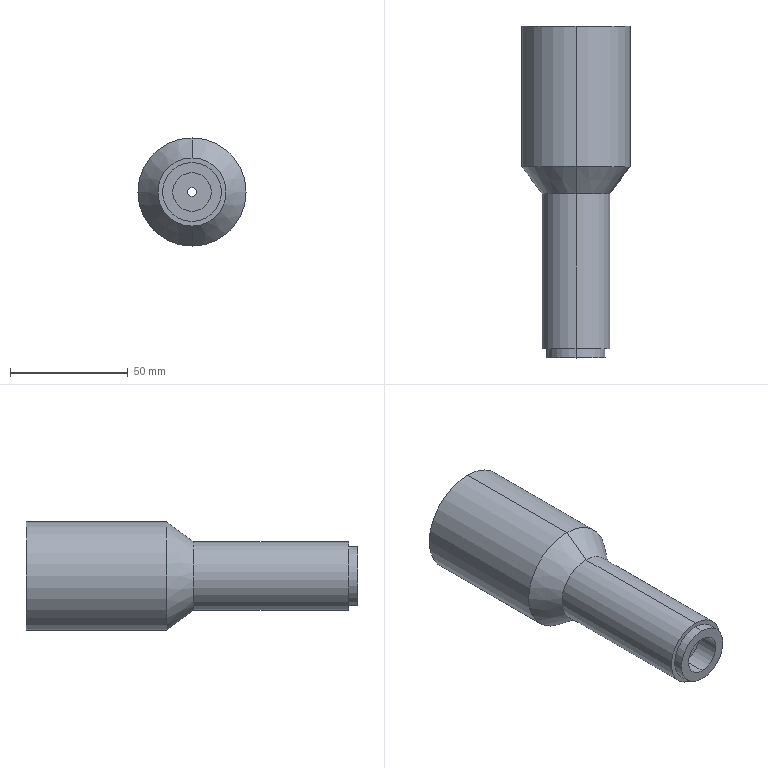Part | STEP file | ASND-0110-Lens | 1 solid | 16 faces | box 46 x 141.1 x 46 mm | volume 154074 mm3 | cylinder 10 | plane 4 | cone 2 | commonest cylinder face diameters 3.74 x2 16.445 x2 25 x2 29 x2 46 x2
STEP:
#1=CARTESIAN_POINT('',(0.,0.,0.));
#2=DIRECTION('',(0.,0.,1.));
#3=DIRECTION('',(1.,0.,0.));
#4=AXIS2_PLACEMENT_3D('',#1,#2,#3);
#5=CARTESIAN_POINT('',(0.,144.654,-23.));
#6=VERTEX_POINT('',#5);
#7=CARTESIAN_POINT('',(0.,144.654,23.));
#8=VERTEX_POINT('',#7);
#9=CARTESIAN_POINT('',(0.,144.654,0.));
#10=DIRECTION('',(0.,-1.,0.));
#11=DIRECTION('',(0.,0.,-1.));
#12=AXIS2_PLACEMENT_3D('',#9,#10,#11);
#13=CIRCLE('',#12,23.);
#14=CARTESIAN_POINT('',(0.,0.,0.));
#15=DIRECTION('',(0.,-1.,0.));
#16=DIRECTION('',(0.,0.,-1.));
#17=AXIS2_PLACEMENT_3D('',#14,#15,#16);
#18=CYLINDRICAL_SURFACE('',#17,23.);
#19=CARTESIAN_POINT('',(0.,-144.654));
#20=DIRECTION('',(1.,0.));
#21=VECTOR('',#20,1.);
#22=LINE('',#19,#21);
#23=(GEOMETRIC_REPRESENTATION_CONTEXT(2)PARAMETRIC_REPRESENTATION_CONTEXT()REPRESENTATION_CONTEXT('',''));
#24=DEFINITIONAL_REPRESENTATION('',(#22),#23);
#25=PCURVE('',#18,#24);
#26=CARTESIAN_POINT('',(23.,144.654,0.));
#27=DIRECTION('',(0.,1.,0.));
#28=DIRECTION('',(0.7071,0.,0.7071));
#29=AXIS2_PLACEMENT_3D('',#26,#27,#28);
#30=PLANE('',#29);
#31=CARTESIAN_POINT('',(-32.527,0.));
#32=CARTESIAN_POINT('',(-4.358,28.169));
#33=CARTESIAN_POINT('',(5.953,-10.311));
#34=CARTESIAN_POINT('',(16.263,-48.79));
#35=CARTESIAN_POINT('',(-22.216,-38.48));
#36=CARTESIAN_POINT('',(-60.696,-28.169));
#37=CARTESIAN_POINT('',(-32.527,0.));
#38=(BOUNDED_CURVE()B_SPLINE_CURVE(2,(#31,#32,#33,#34,#35,#36,#37),.UNSPECIFIED.,.T.,.F.)B_SPLINE_CURVE_WITH_KNOTS((1,2,2,2,2,1),(-2.094,0.,2.094,4.189,6.283,8.378),.UNSPECIFIED.)CURVE()GEOMETRIC_REPRESENTATION_ITEM()RATIONAL_B_SPLINE_CURVE((1.,0.5,1.,0.5,1.,0.5,1.))REPRESENTATION_ITEM(''));
#39=(GEOMETRIC_REPRESENTATION_CONTEXT(2)PARAMETRIC_REPRESENTATION_CONTEXT()REPRESENTATION_CONTEXT('',''));
#40=DEFINITIONAL_REPRESENTATION('',(#38),#39);
#41=PCURVE('',#30,#40);
#42=SURFACE_CURVE('',#13,(#25,#41),.PCURVE_S1.);
#43=EDGE_CURVE('',#6,#8,#42,.T.);
#44=ORIENTED_EDGE('',*,*,#43,.T.);
#45=CARTESIAN_POINT('',(0.,84.922,23.));
#46=VERTEX_POINT('',#45);
#47=CARTESIAN_POINT('',(0.,0.,23.));
#48=DIRECTION('',(0.,-1.,0.));
#49=VECTOR('',#48,1.);
#50=LINE('',#47,#49);
#51=CARTESIAN_POINT('',(3.142,0.));
#52=DIRECTION('',(0.,1.));
#53=VECTOR('',#52,1.);
#54=LINE('',#51,#53);
#55=(GEOMETRIC_REPRESENTATION_CONTEXT(2)PARAMETRIC_REPRESENTATION_CONTEXT()REPRESENTATION_CONTEXT('',''));
#56=DEFINITIONAL_REPRESENTATION('',(#54),#55);
#57=PCURVE('',#18,#56);
#58=CARTESIAN_POINT('',(0.,0.,0.));
#59=DIRECTION('',(0.,-1.,0.));
#60=DIRECTION('',(0.,0.,-1.));
#61=AXIS2_PLACEMENT_3D('',#58,#59,#60);
#62=CYLINDRICAL_SURFACE('',#61,23.);
#63=CARTESIAN_POINT('',(3.142,0.));
#64=DIRECTION('',(0.,1.));
#65=VECTOR('',#64,1.);
#66=LINE('',#63,#65);
#67=(GEOMETRIC_REPRESENTATION_CONTEXT(2)PARAMETRIC_REPRESENTATION_CONTEXT()REPRESENTATION_CONTEXT('',''));
#68=DEFINITIONAL_REPRESENTATION('',(#66),#67);
#69=PCURVE('',#62,#68);
#70=SURFACE_CURVE('',#50,(#57,#69),.PCURVE_S1.);
#71=EDGE_CURVE('',#8,#46,#70,.T.);
#72=ORIENTED_EDGE('',*,*,#71,.T.);
#73=CARTESIAN_POINT('',(0.,84.922,-23.));
#74=VERTEX_POINT('',#73);
#75=CARTESIAN_POINT('',(0.,84.922,0.));
#76=DIRECTION('',(0.,-1.,0.));
#77=DIRECTION('',(0.,0.,-1.));
#78=AXIS2_PLACEMENT_3D('',#75,#76,#77);
#79=CIRCLE('',#78,23.);
#80=CARTESIAN_POINT('',(0.,-84.922));
#81=DIRECTION('',(1.,0.));
#82=VECTOR('',#81,1.);
#83=LINE('',#80,#82);
#84=(GEOMETRIC_REPRESENTATION_CONTEXT(2)PARAMETRIC_REPRESENTATION_CONTEXT()REPRESENTATION_CONTEXT('',''));
#85=DEFINITIONAL_REPRESENTATION('',(#83),#84);
#86=PCURVE('',#18,#85);
#87=CARTESIAN_POINT('',(0.,73.422,0.));
#88=DIRECTION('',(0.,1.,0.));
#89=DIRECTION('',(0.,0.,1.));
#90=AXIS2_PLACEMENT_3D('',#87,#88,#89);
#91=CONICAL_SURFACE('',#90,14.5,0.6365);
#92=CARTESIAN_POINT('',(3.142,11.5));
#93=DIRECTION('',(-1.,0.));
#94=VECTOR('',#93,1.);
#95=LINE('',#92,#94);
#96=(GEOMETRIC_REPRESENTATION_CONTEXT(2)PARAMETRIC_REPRESENTATION_CONTEXT()REPRESENTATION_CONTEXT('',''));
#97=DEFINITIONAL_REPRESENTATION('',(#95),#96);
#98=PCURVE('',#91,#97);
#99=SURFACE_CURVE('',#79,(#86,#98),.PCURVE_S1.);
#100=EDGE_CURVE('',#74,#46,#99,.T.);
#101=ORIENTED_EDGE('',*,*,#100,.F.);
#102=CARTESIAN_POINT('',(0.,0.,-23.));
#103=DIRECTION('',(0.,-1.,0.));
#104=VECTOR('',#103,1.);
#105=LINE('',#102,#104);
#106=CARTESIAN_POINT('',(0.,0.));
#107=DIRECTION('',(0.,1.));
#108=VECTOR('',#107,1.);
#109=LINE('',#106,#108);
#110=(GEOMETRIC_REPRESENTATION_CONTEXT(2)PARAMETRIC_REPRESENTATION_CONTEXT()REPRESENTATION_CONTEXT('',''));
#111=DEFINITIONAL_REPRESENTATION('',(#109),#110);
#112=PCURVE('',#18,#111);
#113=CARTESIAN_POINT('',(6.283,0.));
#114=DIRECTION('',(0.,1.));
#115=VECTOR('',#114,1.);
#116=LINE('',#113,#115);
#117=(GEOMETRIC_REPRESENTATION_CONTEXT(2)PARAMETRIC_REPRESENTATION_CONTEXT()REPRESENTATION_CONTEXT('',''));
#118=DEFINITIONAL_REPRESENTATION('',(#116),#117);
#119=PCURVE('',#62,#118);
#120=SURFACE_CURVE('',#105,(#112,#119),.PCURVE_S1.);
#121=EDGE_CURVE('',#6,#74,#120,.T.);
#122=ORIENTED_EDGE('',*,*,#121,.F.);
#123=EDGE_LOOP('',(#44,#72,#101,#122));
#124=FACE_BOUND('',#123,.T.);
#125=ADVANCED_FACE('',(#124),#18,.T.);
#126=CARTESIAN_POINT('',(0.,73.422,-14.5));
#127=VERTEX_POINT('',#126);
#128=CARTESIAN_POINT('',(0.,73.422,14.5));
#129=VERTEX_POINT('',#128);
#130=CARTESIAN_POINT('',(0.,73.422,0.));
#131=DIRECTION('',(0.,-1.,0.));
#132=DIRECTION('',(0.,0.,-1.));
#133=AXIS2_PLACEMENT_3D('',#130,#131,#132);
#134=CIRCLE('',#133,14.5);
#135=CARTESIAN_POINT('',(3.142,0.));
#136=DIRECTION('',(-1.,0.));
#137=VECTOR('',#136,1.);
#138=LINE('',#135,#137);
#139=(GEOMETRIC_REPRESENTATION_CONTEXT(2)PARAMETRIC_REPRESENTATION_CONTEXT()REPRESENTATION_CONTEXT('',''));
#140=DEFINITIONAL_REPRESENTATION('',(#138),#139);
#141=PCURVE('',#91,#140);
#142=CARTESIAN_POINT('',(0.,0.,0.));
#143=DIRECTION('',(0.,-1.,0.));
#144=DIRECTION('',(0.,0.,-1.));
#145=AXIS2_PLACEMENT_3D('',#142,#143,#144);
#146=CYLINDRICAL_SURFACE('',#145,14.5);
#147=CARTESIAN_POINT('',(0.,-73.422));
#148=DIRECTION('',(1.,0.));
#149=VECTOR('',#148,1.);
#150=LINE('',#147,#149);
#151=(GEOMETRIC_REPRESENTATION_CONTEXT(2)PARAMETRIC_REPRESENTATION_CONTEXT()REPRESENTATION_CONTEXT('',''));
#152=DEFINITIONAL_REPRESENTATION('',(#150),#151);
#153=PCURVE('',#146,#152);
#154=SURFACE_CURVE('',#134,(#141,#153),.PCURVE_S1.);
#155=EDGE_CURVE('',#127,#129,#154,.T.);
#156=ORIENTED_EDGE('',*,*,#155,.F.);
#157=CARTESIAN_POINT('',(0.,73.422,-14.5));
#158=DIRECTION('',(0.,0.8042,-0.5944));
#159=VECTOR('',#158,1.);
#160=LINE('',#157,#159);
#161=CARTESIAN_POINT('',(3.142,0.));
#162=DIRECTION('',(0.,1.));
#163=VECTOR('',#162,1.);
#164=LINE('',#161,#163);
#165=(GEOMETRIC_REPRESENTATION_CONTEXT(2)PARAMETRIC_REPRESENTATION_CONTEXT()REPRESENTATION_CONTEXT('',''));
#166=DEFINITIONAL_REPRESENTATION('',(#164),#165);
#167=PCURVE('',#91,#166);
#168=CARTESIAN_POINT('',(0.,73.422,0.));
#169=DIRECTION('',(0.,1.,0.));
#170=DIRECTION('',(0.,0.,1.));
#171=AXIS2_PLACEMENT_3D('',#168,#169,#170);
#172=CONICAL_SURFACE('',#171,14.5,0.6365);
#173=CARTESIAN_POINT('',(3.142,0.));
#174=DIRECTION('',(0.,1.));
#175=VECTOR('',#174,1.);
#176=LINE('',#173,#175);
#177=(GEOMETRIC_REPRESENTATION_CONTEXT(2)PARAMETRIC_REPRESENTATION_CONTEXT()REPRESENTATION_CONTEXT('',''));
#178=DEFINITIONAL_REPRESENTATION('',(#176),#177);
#179=PCURVE('',#172,#178);
#180=SURFACE_CURVE('',#160,(#167,#179),.PCURVE_S1.);
#181=EDGE_CURVE('',#127,#74,#180,.T.);
#182=ORIENTED_EDGE('',*,*,#181,.T.);
#183=ORIENTED_EDGE('',*,*,#100,.T.);
#184=CARTESIAN_POINT('',(0.,73.422,14.5));
#185=DIRECTION('',(0.,0.8042,0.5944));
#186=VECTOR('',#185,1.);
#187=LINE('',#184,#186);
#188=CARTESIAN_POINT('',(0.,0.));
#189=DIRECTION('',(0.,1.));
#190=VECTOR('',#189,1.);
#191=LINE('',#188,#190);
#192=(GEOMETRIC_REPRESENTATION_CONTEXT(2)PARAMETRIC_REPRESENTATION_CONTEXT()REPRESENTATION_CONTEXT('',''));
#193=DEFINITIONAL_REPRESENTATION('',(#191),#192);
#194=PCURVE('',#91,#193);
#195=CARTESIAN_POINT('',(6.283,0.));
#196=DIRECTION('',(0.,1.));
#197=VECTOR('',#196,1.);
#198=LINE('',#195,#197);
#199=(GEOMETRIC_REPRESENTATION_CONTEXT(2)PARAMETRIC_REPRESENTATION_CONTEXT()REPRESENTATION_CONTEXT('',''));
#200=DEFINITIONAL_REPRESENTATION('',(#198),#199);
#201=PCURVE('',#172,#200);
#202=SURFACE_CURVE('',#187,(#194,#201),.PCURVE_S1.);
#203=EDGE_CURVE('',#129,#46,#202,.T.);
#204=ORIENTED_EDGE('',*,*,#203,.F.);
#205=EDGE_LOOP('',(#156,#182,#183,#204));
#206=FACE_BOUND('',#205,.T.);
#207=ADVANCED_FACE('',(#206),#91,.T.);
#208=ORIENTED_EDGE('',*,*,#155,.T.);
#209=CARTESIAN_POINT('',(0.,7.554,14.5));
#210=VERTEX_POINT('',#209);
#211=CARTESIAN_POINT('',(0.,0.,14.5));
#212=DIRECTION('',(0.,-1.,0.));
#213=VECTOR('',#212,1.);
#214=LINE('',#211,#213);
#215=CARTESIAN_POINT('',(3.142,0.));
#216=DIRECTION('',(0.,1.));
#217=VECTOR('',#216,1.);
#218=LINE('',#215,#217);
#219=(GEOMETRIC_REPRESENTATION_CONTEXT(2)PARAMETRIC_REPRESENTATION_CONTEXT()REPRESENTATION_CONTEXT('',''));
#220=DEFINITIONAL_REPRESENTATION('',(#218),#219);
#221=PCURVE('',#146,#220);
#222=CARTESIAN_POINT('',(0.,0.,0.));
#223=DIRECTION('',(0.,-1.,0.));
#224=DIRECTION('',(0.,0.,-1.));
#225=AXIS2_PLACEMENT_3D('',#222,#223,#224);
#226=CYLINDRICAL_SURFACE('',#225,14.5);
#227=CARTESIAN_POINT('',(3.142,0.));
#228=DIRECTION('',(0.,1.));
#229=VECTOR('',#228,1.);
#230=LINE('',#227,#229);
#231=(GEOMETRIC_REPRESENTATION_CONTEXT(2)PARAMETRIC_REPRESENTATION_CONTEXT()REPRESENTATION_CONTEXT('',''));
#232=DEFINITIONAL_REPRESENTATION('',(#230),#231);
#233=PCURVE('',#226,#232);
#234=SURFACE_CURVE('',#214,(#221,#233),.PCURVE_S1.);
#235=EDGE_CURVE('',#129,#210,#234,.T.);
#236=ORIENTED_EDGE('',*,*,#235,.T.);
#237=CARTESIAN_POINT('',(0.,7.554,-14.5));
#238=VERTEX_POINT('',#237);
#239=CARTESIAN_POINT('',(0.,7.554,0.));
#240=DIRECTION('',(0.,-1.,0.));
#241=DIRECTION('',(0.,0.,-1.));
#242=AXIS2_PLACEMENT_3D('',#239,#240,#241);
#243=CIRCLE('',#242,14.5);
#244=CARTESIAN_POINT('',(0.,-7.554));
#245=DIRECTION('',(1.,0.));
#246=VECTOR('',#245,1.);
#247=LINE('',#244,#246);
#248=(GEOMETRIC_REPRESENTATION_CONTEXT(2)PARAMETRIC_REPRESENTATION_CONTEXT()REPRESENTATION_CONTEXT('',''));
#249=DEFINITIONAL_REPRESENTATION('',(#247),#248);
#250=PCURVE('',#146,#249);
#251=CARTESIAN_POINT('',(14.5,7.554,0.));
#252=DIRECTION('',(0.,-1.,0.));
#253=DIRECTION('',(0.7071,0.,0.7071));
#254=AXIS2_PLACEMENT_3D('',#251,#252,#253);
#255=PLANE('',#254);
#256=CARTESIAN_POINT('',(-10.253,10.253));
#257=DIRECTION('',(-0.7071,-0.7071));
#258=AXIS2_PLACEMENT_2D('',#256,#257);
#259=CIRCLE('',#258,14.5);
#260=(GEOMETRIC_REPRESENTATION_CONTEXT(2)PARAMETRIC_REPRESENTATION_CONTEXT()REPRESENTATION_CONTEXT('',''));
#261=DEFINITIONAL_REPRESENTATION('',(#259),#260);
#262=PCURVE('',#255,#261);
#263=SURFACE_CURVE('',#243,(#250,#262),.PCURVE_S1.);
#264=EDGE_CURVE('',#238,#210,#263,.T.);
#265=ORIENTED_EDGE('',*,*,#264,.F.);
#266=CARTESIAN_POINT('',(0.,0.,-14.5));
#267=DIRECTION('',(0.,-1.,0.));
#268=VECTOR('',#267,1.);
#269=LINE('',#266,#268);
#270=CARTESIAN_POINT('',(0.,0.));
#271=DIRECTION('',(0.,1.));
#272=VECTOR('',#271,1.);
#273=LINE('',#270,#272);
#274=(GEOMETRIC_REPRESENTATION_CONTEXT(2)PARAMETRIC_REPRESENTATION_CONTEXT()REPRESENTATION_CONTEXT('',''));
#275=DEFINITIONAL_REPRESENTATION('',(#273),#274);
#276=PCURVE('',#146,#275);
#277=CARTESIAN_POINT('',(6.283,0.));
#278=DIRECTION('',(0.,1.));
#279=VECTOR('',#278,1.);
#280=LINE('',#277,#279);
#281=(GEOMETRIC_REPRESENTATION_CONTEXT(2)PARAMETRIC_REPRESENTATION_CONTEXT()REPRESENTATION_CONTEXT('',''));
#282=DEFINITIONAL_REPRESENTATION('',(#280),#281);
#283=PCURVE('',#226,#282);
#284=SURFACE_CURVE('',#269,(#276,#283),.PCURVE_S1.);
#285=EDGE_CURVE('',#127,#238,#284,.T.);
#286=ORIENTED_EDGE('',*,*,#285,.F.);
#287=EDGE_LOOP('',(#208,#236,#265,#286));
#288=FACE_BOUND('',#287,.T.);
#289=ADVANCED_FACE('',(#288),#146,.T.);
#290=CARTESIAN_POINT('',(0.,7.554,-12.5));
#291=VERTEX_POINT('',#290);
#292=CARTESIAN_POINT('',(0.,7.554,12.5));
#293=VERTEX_POINT('',#292);
#294=CARTESIAN_POINT('',(0.,7.554,0.));
#295=DIRECTION('',(0.,-1.,0.));
#296=DIRECTION('',(0.,0.,-1.));
#297=AXIS2_PLACEMENT_3D('',#294,#295,#296);
#298=CIRCLE('',#297,12.5);
#299=CARTESIAN_POINT('',(0.,0.,0.));
#300=DIRECTION('',(0.,-1.,0.));
#301=DIRECTION('',(0.,0.,-1.));
#302=AXIS2_PLACEMENT_3D('',#299,#300,#301);
#303=CYLINDRICAL_SURFACE('',#302,12.5);
#304=CARTESIAN_POINT('',(0.,-7.554));
#305=DIRECTION('',(1.,0.));
#306=VECTOR('',#305,1.);
#307=LINE('',#304,#306);
#308=(GEOMETRIC_REPRESENTATION_CONTEXT(2)PARAMETRIC_REPRESENTATION_CONTEXT()REPRESENTATION_CONTEXT('',''));
#309=DEFINITIONAL_REPRESENTATION('',(#307),#308);
#310=PCURVE('',#303,#309);
#311=CARTESIAN_POINT('',(-10.253,10.253));
#312=DIRECTION('',(-0.7071,-0.7071));
#313=AXIS2_PLACEMENT_2D('',#311,#312);
#314=CIRCLE('',#313,12.5);
#315=(GEOMETRIC_REPRESENTATION_CONTEXT(2)PARAMETRIC_REPRESENTATION_CONTEXT()REPRESENTATION_CONTEXT('',''));
#316=DEFINITIONAL_REPRESENTATION('',(#314),#315);
#317=PCURVE('',#255,#316);
#318=SURFACE_CURVE('',#298,(#310,#317),.PCURVE_S1.);
#319=EDGE_CURVE('',#291,#293,#318,.T.);
#320=ORIENTED_EDGE('',*,*,#319,.T.);
#321=CARTESIAN_POINT('',(0.,3.554,12.5));
#322=VERTEX_POINT('',#321);
#323=CARTESIAN_POINT('',(0.,0.,12.5));
#324=DIRECTION('',(0.,-1.,0.));
#325=VECTOR('',#324,1.);
#326=LINE('',#323,#325);
#327=CARTESIAN_POINT('',(3.142,0.));
#328=DIRECTION('',(0.,1.));
#329=VECTOR('',#328,1.);
#330=LINE('',#327,#329);
#331=(GEOMETRIC_REPRESENTATION_CONTEXT(2)PARAMETRIC_REPRESENTATION_CONTEXT()REPRESENTATION_CONTEXT('',''));
#332=DEFINITIONAL_REPRESENTATION('',(#330),#331);
#333=PCURVE('',#303,#332);
#334=CARTESIAN_POINT('',(0.,0.,0.));
#335=DIRECTION('',(0.,-1.,0.));
#336=DIRECTION('',(0.,0.,-1.));
#337=AXIS2_PLACEMENT_3D('',#334,#335,#336);
#338=CYLINDRICAL_SURFACE('',#337,12.5);
#339=CARTESIAN_POINT('',(3.142,0.));
#340=DIRECTION('',(0.,1.));
#341=VECTOR('',#340,1.);
#342=LINE('',#339,#341);
#343=(GEOMETRIC_REPRESENTATION_CONTEXT(2)PARAMETRIC_REPRESENTATION_CONTEXT()REPRESENTATION_CONTEXT('',''));
#344=DEFINITIONAL_REPRESENTATION('',(#342),#343);
#345=PCURVE('',#338,#344);
#346=SURFACE_CURVE('',#326,(#333,#345),.PCURVE_S1.);
#347=EDGE_CURVE('',#293,#322,#346,.T.);
#348=ORIENTED_EDGE('',*,*,#347,.T.);
#349=CARTESIAN_POINT('',(0.,3.554,-12.5));
#350=VERTEX_POINT('',#349);
#351=CARTESIAN_POINT('',(0.,3.554,0.));
#352=DIRECTION('',(0.,-1.,0.));
#353=DIRECTION('',(0.,0.,-1.));
#354=AXIS2_PLACEMENT_3D('',#351,#352,#353);
#355=CIRCLE('',#354,12.5);
#356=CARTESIAN_POINT('',(0.,-3.554));
#357=DIRECTION('',(1.,0.));
#358=VECTOR('',#357,1.);
#359=LINE('',#356,#358);
#360=(GEOMETRIC_REPRESENTATION_CONTEXT(2)PARAMETRIC_REPRESENTATION_CONTEXT()REPRESENTATION_CONTEXT('',''));
#361=DEFINITIONAL_REPRESENTATION('',(#359),#360);
#362=PCURVE('',#303,#361);
#363=CARTESIAN_POINT('',(12.5,3.554,0.));
#364=DIRECTION('',(0.,-1.,0.));
#365=DIRECTION('',(0.7071,0.,0.7071));
#366=AXIS2_PLACEMENT_3D('',#363,#364,#365);
#367=PLANE('',#366);
#368=CARTESIAN_POINT('',(-8.839,8.839));
#369=DIRECTION('',(-0.7071,-0.7071));
#370=AXIS2_PLACEMENT_2D('',#368,#369);
#371=CIRCLE('',#370,12.5);
#372=(GEOMETRIC_REPRESENTATION_CONTEXT(2)PARAMETRIC_REPRESENTATION_CONTEXT()REPRESENTATION_CONTEXT('',''));
#373=DEFINITIONAL_REPRESENTATION('',(#371),#372);
#374=PCURVE('',#367,#373);
#375=SURFACE_CURVE('',#355,(#362,#374),.PCURVE_S1.);
#376=EDGE_CURVE('',#350,#322,#375,.T.);
#377=ORIENTED_EDGE('',*,*,#376,.F.);
#378=CARTESIAN_POINT('',(0.,0.,-12.5));
#379=DIRECTION('',(0.,-1.,0.));
#380=VECTOR('',#379,1.);
#381=LINE('',#378,#380);
#382=CARTESIAN_POINT('',(0.,0.));
#383=DIRECTION('',(0.,1.));
#384=VECTOR('',#383,1.);
#385=LINE('',#382,#384);
#386=(GEOMETRIC_REPRESENTATION_CONTEXT(2)PARAMETRIC_REPRESENTATION_CONTEXT()REPRESENTATION_CONTEXT('',''));
#387=DEFINITIONAL_REPRESENTATION('',(#385),#386);
#388=PCURVE('',#303,#387);
#389=CARTESIAN_POINT('',(6.283,0.));
#390=DIRECTION('',(0.,1.));
#391=VECTOR('',#390,1.);
#392=LINE('',#389,#391);
#393=(GEOMETRIC_REPRESENTATION_CONTEXT(2)PARAMETRIC_REPRESENTATION_CONTEXT()REPRESENTATION_CONTEXT('',''));
#394=DEFINITIONAL_REPRESENTATION('',(#392),#393);
#395=PCURVE('',#338,#394);
#396=SURFACE_CURVE('',#381,(#388,#395),.PCURVE_S1.);
#397=EDGE_CURVE('',#291,#350,#396,.T.);
#398=ORIENTED_EDGE('',*,*,#397,.F.);
#399=EDGE_LOOP('',(#320,#348,#377,#398));
#400=FACE_BOUND('',#399,.T.);
#401=ADVANCED_FACE('',(#400),#303,.T.);
#402=CARTESIAN_POINT('',(0.,13.654,-8.222));
#403=VERTEX_POINT('',#402);
#404=CARTESIAN_POINT('',(0.,3.554,-8.222));
#405=VERTEX_POINT('',#404);
#406=CARTESIAN_POINT('',(0.,0.,-8.222));
#407=DIRECTION('',(0.,-1.,0.));
#408=VECTOR('',#407,1.);
#409=LINE('',#406,#408);
#410=CARTESIAN_POINT('',(0.,0.,0.));
#411=DIRECTION('',(0.,-1.,0.));
#412=DIRECTION('',(0.,0.,-1.));
#413=AXIS2_PLACEMENT_3D('',#410,#411,#412);
#414=CYLINDRICAL_SURFACE('',#413,8.222);
#415=CARTESIAN_POINT('',(6.283,0.));
#416=DIRECTION('',(0.,1.));
#417=VECTOR('',#416,1.);
#418=LINE('',#415,#417);
#419=(GEOMETRIC_REPRESENTATION_CONTEXT(2)PARAMETRIC_REPRESENTATION_CONTEXT()REPRESENTATION_CONTEXT('',''));
#420=DEFINITIONAL_REPRESENTATION('',(#418),#419);
#421=PCURVE('',#414,#420);
#422=CARTESIAN_POINT('',(0.,0.,0.));
#423=DIRECTION('',(0.,-1.,0.));
#424=DIRECTION('',(0.,0.,-1.));
#425=AXIS2_PLACEMENT_3D('',#422,#423,#424);
#426=CYLINDRICAL_SURFACE('',#425,8.222);
#427=CARTESIAN_POINT('',(0.,0.));
#428=DIRECTION('',(0.,1.));
#429=VECTOR('',#428,1.);
#430=LINE('',#427,#429);
#431=(GEOMETRIC_REPRESENTATION_CONTEXT(2)PARAMETRIC_REPRESENTATION_CONTEXT()REPRESENTATION_CONTEXT('',''));
#432=DEFINITIONAL_REPRESENTATION('',(#430),#431);
#433=PCURVE('',#426,#432);
#434=SURFACE_CURVE('',#409,(#421,#433),.PCURVE_S1.);
#435=EDGE_CURVE('',#403,#405,#434,.T.);
#436=ORIENTED_EDGE('',*,*,#435,.T.);
#437=CARTESIAN_POINT('',(0.,3.554,8.222));
#438=VERTEX_POINT('',#437);
#439=CARTESIAN_POINT('',(0.,3.554,0.));
#440=DIRECTION('',(0.,-1.,0.));
#441=DIRECTION('',(0.,0.,-1.));
#442=AXIS2_PLACEMENT_3D('',#439,#440,#441);
#443=CIRCLE('',#442,8.222);
#444=CARTESIAN_POINT('',(0.,-3.554));
#445=DIRECTION('',(1.,0.));
#446=VECTOR('',#445,1.);
#447=LINE('',#444,#446);
#448=(GEOMETRIC_REPRESENTATION_CONTEXT(2)PARAMETRIC_REPRESENTATION_CONTEXT()REPRESENTATION_CONTEXT('',''));
#449=DEFINITIONAL_REPRESENTATION('',(#447),#448);
#450=PCURVE('',#414,#449);
#451=CARTESIAN_POINT('',(-8.839,8.839));
#452=DIRECTION('',(-0.7071,-0.7071));
#453=AXIS2_PLACEMENT_2D('',#451,#452);
#454=CIRCLE('',#453,8.222);
#455=(GEOMETRIC_REPRESENTATION_CONTEXT(2)PARAMETRIC_REPRESENTATION_CONTEXT()REPRESENTATION_CONTEXT('',''));
#456=DEFINITIONAL_REPRESENTATION('',(#454),#455);
#457=PCURVE('',#367,#456);
#458=SURFACE_CURVE('',#443,(#450,#457),.PCURVE_S1.);
#459=EDGE_CURVE('',#438,#405,#458,.T.);
#460=ORIENTED_EDGE('',*,*,#459,.F.);
#461=CARTESIAN_POINT('',(0.,13.654,8.222));
#462=VERTEX_POINT('',#461);
#463=CARTESIAN_POINT('',(0.,0.,8.222));
#464=DIRECTION('',(0.,-1.,0.));
#465=VECTOR('',#464,1.);
#466=LINE('',#463,#465);
#467=CARTESIAN_POINT('',(3.142,0.));
#468=DIRECTION('',(0.,1.));
#469=VECTOR('',#468,1.);
#470=LINE('',#467,#469);
#471=(GEOMETRIC_REPRESENTATION_CONTEXT(2)PARAMETRIC_REPRESENTATION_CONTEXT()REPRESENTATION_CONTEXT('',''));
#472=DEFINITIONAL_REPRESENTATION('',(#470),#471);
#473=PCURVE('',#414,#472);
#474=CARTESIAN_POINT('',(3.142,0.));
#475=DIRECTION('',(0.,1.));
#476=VECTOR('',#475,1.);
#477=LINE('',#474,#476);
#478=(GEOMETRIC_REPRESENTATION_CONTEXT(2)PARAMETRIC_REPRESENTATION_CONTEXT()REPRESENTATION_CONTEXT('',''));
#479=DEFINITIONAL_REPRESENTATION('',(#477),#478);
#480=PCURVE('',#426,#479);
#481=SURFACE_CURVE('',#466,(#473,#480),.PCURVE_S1.);
#482=EDGE_CURVE('',#462,#438,#481,.T.);
#483=ORIENTED_EDGE('',*,*,#482,.F.);
#484=CARTESIAN_POINT('',(0.,13.654,0.));
#485=DIRECTION('',(0.,-1.,0.));
#486=DIRECTION('',(0.,0.,-1.));
#487=AXIS2_PLACEMENT_3D('',#484,#485,#486);
#488=CIRCLE('',#487,8.222);
#489=CARTESIAN_POINT('',(0.,-13.654));
#490=DIRECTION('',(1.,0.));
#491=VECTOR('',#490,1.);
#492=LINE('',#489,#491);
#493=(GEOMETRIC_REPRESENTATION_CONTEXT(2)PARAMETRIC_REPRESENTATION_CONTEXT()REPRESENTATION_CONTEXT('',''));
#494=DEFINITIONAL_REPRESENTATION('',(#492),#493);
#495=PCURVE('',#414,#494);
#496=CARTESIAN_POINT('',(1.87,13.654,0.));
#497=DIRECTION('',(0.,-1.,0.));
#498=DIRECTION('',(0.7071,0.,0.7071));
#499=AXIS2_PLACEMENT_3D('',#496,#497,#498);
#500=PLANE('',#499);
#501=CARTESIAN_POINT('',(-1.322,1.322));
#502=DIRECTION('',(-0.7071,-0.7071));
#503=AXIS2_PLACEMENT_2D('',#501,#502);
#504=CIRCLE('',#503,8.222);
#505=(GEOMETRIC_REPRESENTATION_CONTEXT(2)PARAMETRIC_REPRESENTATION_CONTEXT()REPRESENTATION_CONTEXT('',''));
#506=DEFINITIONAL_REPRESENTATION('',(#504),#505);
#507=PCURVE('',#500,#506);
#508=SURFACE_CURVE('',#488,(#495,#507),.PCURVE_S1.);
#509=EDGE_CURVE('',#462,#403,#508,.T.);
#510=ORIENTED_EDGE('',*,*,#509,.T.);
#511=EDGE_LOOP('',(#436,#460,#483,#510));
#512=FACE_BOUND('',#511,.F.);
#513=ADVANCED_FACE('',(#512),#414,.F.);
#514=CARTESIAN_POINT('',(0.,144.654,-1.87));
#515=VERTEX_POINT('',#514);
#516=CARTESIAN_POINT('',(0.,13.654,-1.87));
#517=VERTEX_POINT('',#516);
#518=CARTESIAN_POINT('',(0.,0.,-1.87));
#519=DIRECTION('',(0.,-1.,0.));
#520=VECTOR('',#519,1.);
#521=LINE('',#518,#520);
#522=CARTESIAN_POINT('',(0.,0.,0.));
#523=DIRECTION('',(0.,-1.,0.));
#524=DIRECTION('',(0.,0.,-1.));
#525=AXIS2_PLACEMENT_3D('',#522,#523,#524);
#526=CYLINDRICAL_SURFACE('',#525,1.87);
#527=CARTESIAN_POINT('',(6.283,0.));
#528=DIRECTION('',(0.,1.));
#529=VECTOR('',#528,1.);
#530=LINE('',#527,#529);
#531=(GEOMETRIC_REPRESENTATION_CONTEXT(2)PARAMETRIC_REPRESENTATION_CONTEXT()REPRESENTATION_CONTEXT('',''));
#532=DEFINITIONAL_REPRESENTATION('',(#530),#531);
#533=PCURVE('',#526,#532);
#534=CARTESIAN_POINT('',(0.,0.,0.));
#535=DIRECTION('',(0.,-1.,0.));
#536=DIRECTION('',(0.,0.,-1.));
#537=AXIS2_PLACEMENT_3D('',#534,#535,#536);
#538=CYLINDRICAL_SURFACE('',#537,1.87);
#539=CARTESIAN_POINT('',(0.,0.));
#540=DIRECTION('',(0.,1.));
#541=VECTOR('',#540,1.);
#542=LINE('',#539,#541);
#543=(GEOMETRIC_REPRESENTATION_CONTEXT(2)PARAMETRIC_REPRESENTATION_CONTEXT()REPRESENTATION_CONTEXT('',''));
#544=DEFINITIONAL_REPRESENTATION('',(#542),#543);
#545=PCURVE('',#538,#544);
#546=SURFACE_CURVE('',#521,(#533,#545),.PCURVE_S1.);
#547=EDGE_CURVE('',#515,#517,#546,.T.);
#548=ORIENTED_EDGE('',*,*,#547,.T.);
#549=CARTESIAN_POINT('',(0.,13.654,1.87));
#550=VERTEX_POINT('',#549);
#551=CARTESIAN_POINT('',(0.,13.654,0.));
#552=DIRECTION('',(0.,-1.,0.));
#553=DIRECTION('',(0.,0.,-1.));
#554=AXIS2_PLACEMENT_3D('',#551,#552,#553);
#555=CIRCLE('',#554,1.87);
#556=CARTESIAN_POINT('',(0.,-13.654));
#557=DIRECTION('',(1.,0.));
#558=VECTOR('',#557,1.);
#559=LINE('',#556,#558);
#560=(GEOMETRIC_REPRESENTATION_CONTEXT(2)PARAMETRIC_REPRESENTATION_CONTEXT()REPRESENTATION_CONTEXT('',''));
#561=DEFINITIONAL_REPRESENTATION('',(#559),#560);
#562=PCURVE('',#526,#561);
#563=CARTESIAN_POINT('',(-1.322,1.322));
#564=DIRECTION('',(-0.7071,-0.7071));
#565=AXIS2_PLACEMENT_2D('',#563,#564);
#566=CIRCLE('',#565,1.87);
#567=(GEOMETRIC_REPRESENTATION_CONTEXT(2)PARAMETRIC_REPRESENTATION_CONTEXT()REPRESENTATION_CONTEXT('',''));
#568=DEFINITIONAL_REPRESENTATION('',(#566),#567);
#569=PCURVE('',#500,#568);
#570=SURFACE_CURVE('',#555,(#562,#569),.PCURVE_S1.);
#571=EDGE_CURVE('',#550,#517,#570,.T.);
#572=ORIENTED_EDGE('',*,*,#571,.F.);
#573=CARTESIAN_POINT('',(0.,144.654,1.87));
#574=VERTEX_POINT('',#573);
#575=CARTESIAN_POINT('',(0.,0.,1.87));
#576=DIRECTION('',(0.,-1.,0.));
#577=VECTOR('',#576,1.);
#578=LINE('',#575,#577);
#579=CARTESIAN_POINT('',(3.142,0.));
#580=DIRECTION('',(0.,1.));
#581=VECTOR('',#580,1.);
#582=LINE('',#579,#581);
#583=(GEOMETRIC_REPRESENTATION_CONTEXT(2)PARAMETRIC_REPRESENTATION_CONTEXT()REPRESENTATION_CONTEXT('',''));
#584=DEFINITIONAL_REPRESENTATION('',(#582),#583);
#585=PCURVE('',#526,#584);
#586=CARTESIAN_POINT('',(3.142,0.));
#587=DIRECTION('',(0.,1.));
#588=VECTOR('',#587,1.);
#589=LINE('',#586,#588);
#590=(GEOMETRIC_REPRESENTATION_CONTEXT(2)PARAMETRIC_REPRESENTATION_CONTEXT()REPRESENTATION_CONTEXT('',''));
#591=DEFINITIONAL_REPRESENTATION('',(#589),#590);
#592=PCURVE('',#538,#591);
#593=SURFACE_CURVE('',#578,(#585,#592),.PCURVE_S1.);
#594=EDGE_CURVE('',#574,#550,#593,.T.);
#595=ORIENTED_EDGE('',*,*,#594,.F.);
#596=CARTESIAN_POINT('',(0.,144.654,0.));
#597=DIRECTION('',(0.,-1.,0.));
#598=DIRECTION('',(0.,0.,-1.));
#599=AXIS2_PLACEMENT_3D('',#596,#597,#598);
#600=CIRCLE('',#599,1.87);
#601=CARTESIAN_POINT('',(0.,-144.654));
#602=DIRECTION('',(1.,0.));
#603=VECTOR('',#602,1.);
#604=LINE('',#601,#603);
#605=(GEOMETRIC_REPRESENTATION_CONTEXT(2)PARAMETRIC_REPRESENTATION_CONTEXT()REPRESENTATION_CONTEXT('',''));
#606=DEFINITIONAL_REPRESENTATION('',(#604),#605);
#607=PCURVE('',#526,#606);
#608=CARTESIAN_POINT('',(-17.586,-14.941));
#609=CARTESIAN_POINT('',(-15.295,-12.651));
#610=CARTESIAN_POINT('',(-14.457,-15.779));
#611=CARTESIAN_POINT('',(-13.619,-18.908));
#612=CARTESIAN_POINT('',(-16.747,-18.07));
#613=CARTESIAN_POINT('',(-19.876,-17.231));
#614=CARTESIAN_POINT('',(-17.586,-14.941));
#615=(BOUNDED_CURVE()B_SPLINE_CURVE(2,(#608,#609,#610,#611,#612,#613,#614),.UNSPECIFIED.,.T.,.F.)B_SPLINE_CURVE_WITH_KNOTS((1,2,2,2,2,1),(-2.094,0.,2.094,4.189,6.283,8.378),.UNSPECIFIED.)CURVE()GEOMETRIC_REPRESENTATION_ITEM()RATIONAL_B_SPLINE_CURVE((1.,0.5,1.,0.5,1.,0.5,1.))REPRESENTATION_ITEM(''));
#616=(GEOMETRIC_REPRESENTATION_CONTEXT(2)PARAMETRIC_REPRESENTATION_CONTEXT()REPRESENTATION_CONTEXT('',''));
#617=DEFINITIONAL_REPRESENTATION('',(#615),#616);
#618=PCURVE('',#30,#617);
#619=SURFACE_CURVE('',#600,(#607,#618),.PCURVE_S1.);
#620=EDGE_CURVE('',#574,#515,#619,.T.);
#621=ORIENTED_EDGE('',*,*,#620,.T.);
#622=EDGE_LOOP('',(#548,#572,#595,#621));
#623=FACE_BOUND('',#622,.F.);
#624=ADVANCED_FACE('',(#623),#526,.F.);
#625=CARTESIAN_POINT('',(0.,13.654,0.));
#626=DIRECTION('',(0.,-1.,0.));
#627=DIRECTION('',(0.,0.,-1.));
#628=AXIS2_PLACEMENT_3D('',#625,#626,#627);
#629=CIRCLE('',#628,1.87);
#630=CARTESIAN_POINT('',(0.,-13.654));
#631=DIRECTION('',(1.,0.));
#632=VECTOR('',#631,1.);
#633=LINE('',#630,#632);
#634=(GEOMETRIC_REPRESENTATION_CONTEXT(2)PARAMETRIC_REPRESENTATION_CONTEXT()REPRESENTATION_CONTEXT('',''));
#635=DEFINITIONAL_REPRESENTATION('',(#633),#634);
#636=PCURVE('',#538,#635);
#637=CARTESIAN_POINT('',(-1.322,1.322));
#638=DIRECTION('',(-0.7071,-0.7071));
#639=AXIS2_PLACEMENT_2D('',#637,#638);
#640=CIRCLE('',#639,1.87);
#641=(GEOMETRIC_REPRESENTATION_CONTEXT(2)PARAMETRIC_REPRESENTATION_CONTEXT()REPRESENTATION_CONTEXT('',''));
#642=DEFINITIONAL_REPRESENTATION('',(#640),#641);
#643=PCURVE('',#500,#642);
#644=SURFACE_CURVE('',#629,(#636,#643),.PCURVE_S1.);
#645=EDGE_CURVE('',#517,#550,#644,.T.);
#646=ORIENTED_EDGE('',*,*,#645,.F.);
#647=ORIENTED_EDGE('',*,*,#547,.F.);
#648=CARTESIAN_POINT('',(0.,144.654,0.));
#649=DIRECTION('',(0.,-1.,0.));
#650=DIRECTION('',(0.,0.,-1.));
#651=AXIS2_PLACEMENT_3D('',#648,#649,#650);
#652=CIRCLE('',#651,1.87);
#653=CARTESIAN_POINT('',(0.,-144.654));
#654=DIRECTION('',(1.,0.));
#655=VECTOR('',#654,1.);
#656=LINE('',#653,#655);
#657=(GEOMETRIC_REPRESENTATION_CONTEXT(2)PARAMETRIC_REPRESENTATION_CONTEXT()REPRESENTATION_CONTEXT('',''));
#658=DEFINITIONAL_REPRESENTATION('',(#656),#657);
#659=PCURVE('',#538,#658);
#660=CARTESIAN_POINT('',(-17.586,-14.941));
#661=CARTESIAN_POINT('',(-15.295,-12.651));
#662=CARTESIAN_POINT('',(-14.457,-15.779));
#663=CARTESIAN_POINT('',(-13.619,-18.908));
#664=CARTESIAN_POINT('',(-16.747,-18.07));
#665=CARTESIAN_POINT('',(-19.876,-17.231));
#666=CARTESIAN_POINT('',(-17.586,-14.941));
#667=(BOUNDED_CURVE()B_SPLINE_CURVE(2,(#660,#661,#662,#663,#664,#665,#666),.UNSPECIFIED.,.T.,.F.)B_SPLINE_CURVE_WITH_KNOTS((1,2,2,2,2,1),(-2.094,0.,2.094,4.189,6.283,8.378),.UNSPECIFIED.)CURVE()GEOMETRIC_REPRESENTATION_ITEM()RATIONAL_B_SPLINE_CURVE((1.,0.5,1.,0.5,1.,0.5,1.))REPRESENTATION_ITEM(''));
#668=(GEOMETRIC_REPRESENTATION_CONTEXT(2)PARAMETRIC_REPRESENTATION_CONTEXT()REPRESENTATION_CONTEXT('',''));
#669=DEFINITIONAL_REPRESENTATION('',(#667),#668);
#670=PCURVE('',#30,#669);
#671=SURFACE_CURVE('',#652,(#659,#670),.PCURVE_S1.);
#672=EDGE_CURVE('',#515,#574,#671,.T.);
#673=ORIENTED_EDGE('',*,*,#672,.T.);
#674=ORIENTED_EDGE('',*,*,#594,.T.);
#675=EDGE_LOOP('',(#646,#647,#673,#674));
#676=FACE_BOUND('',#675,.F.);
#677=ADVANCED_FACE('',(#676),#538,.F.);
#678=CARTESIAN_POINT('',(0.,13.654,0.));
#679=DIRECTION('',(0.,-1.,0.));
#680=DIRECTION('',(0.,0.,-1.));
#681=AXIS2_PLACEMENT_3D('',#678,#679,#680);
#682=CIRCLE('',#681,8.222);
#683=CARTESIAN_POINT('',(-1.322,1.322));
#684=DIRECTION('',(-0.7071,-0.7071));
#685=AXIS2_PLACEMENT_2D('',#683,#684);
#686=CIRCLE('',#685,8.222);
#687=(GEOMETRIC_REPRESENTATION_CONTEXT(2)PARAMETRIC_REPRESENTATION_CONTEXT()REPRESENTATION_CONTEXT('',''));
#688=DEFINITIONAL_REPRESENTATION('',(#686),#687);
#689=PCURVE('',#500,#688);
#690=CARTESIAN_POINT('',(0.,-13.654));
#691=DIRECTION('',(1.,0.));
#692=VECTOR('',#691,1.);
#693=LINE('',#690,#692);
#694=(GEOMETRIC_REPRESENTATION_CONTEXT(2)PARAMETRIC_REPRESENTATION_CONTEXT()REPRESENTATION_CONTEXT('',''));
#695=DEFINITIONAL_REPRESENTATION('',(#693),#694);
#696=PCURVE('',#426,#695);
#697=SURFACE_CURVE('',#682,(#689,#696),.PCURVE_S1.);
#698=EDGE_CURVE('',#403,#462,#697,.T.);
#699=ORIENTED_EDGE('',*,*,#698,.T.);
#700=ORIENTED_EDGE('',*,*,#509,.T.);
#701=EDGE_LOOP('',(#699,#700));
#702=FACE_BOUND('',#701,.T.);
#703=ORIENTED_EDGE('',*,*,#645,.F.);
#704=ORIENTED_EDGE('',*,*,#571,.F.);
#705=EDGE_LOOP('',(#703,#704));
#706=FACE_BOUND('',#705,.T.);
#707=ADVANCED_FACE('',(#702,#706),#500,.T.);
#708=CARTESIAN_POINT('',(0.,3.554,0.));
#709=DIRECTION('',(0.,-1.,0.));
#710=DIRECTION('',(0.,0.,-1.));
#711=AXIS2_PLACEMENT_3D('',#708,#709,#710);
#712=CIRCLE('',#711,8.222);
#713=CARTESIAN_POINT('',(0.,-3.554));
#714=DIRECTION('',(1.,0.));
#715=VECTOR('',#714,1.);
#716=LINE('',#713,#715);
#717=(GEOMETRIC_REPRESENTATION_CONTEXT(2)PARAMETRIC_REPRESENTATION_CONTEXT()REPRESENTATION_CONTEXT('',''));
#718=DEFINITIONAL_REPRESENTATION('',(#716),#717);
#719=PCURVE('',#426,#718);
#720=CARTESIAN_POINT('',(-8.839,8.839));
#721=DIRECTION('',(-0.7071,-0.7071));
#722=AXIS2_PLACEMENT_2D('',#720,#721);
#723=CIRCLE('',#722,8.222);
#724=(GEOMETRIC_REPRESENTATION_CONTEXT(2)PARAMETRIC_REPRESENTATION_CONTEXT()REPRESENTATION_CONTEXT('',''));
#725=DEFINITIONAL_REPRESENTATION('',(#723),#724);
#726=PCURVE('',#367,#725);
#727=SURFACE_CURVE('',#712,(#719,#726),.PCURVE_S1.);
#728=EDGE_CURVE('',#405,#438,#727,.T.);
#729=ORIENTED_EDGE('',*,*,#728,.F.);
#730=ORIENTED_EDGE('',*,*,#435,.F.);
#731=ORIENTED_EDGE('',*,*,#698,.T.);
#732=ORIENTED_EDGE('',*,*,#482,.T.);
#733=EDGE_LOOP('',(#729,#730,#731,#732));
#734=FACE_BOUND('',#733,.F.);
#735=ADVANCED_FACE('',(#734),#426,.F.);
#736=ORIENTED_EDGE('',*,*,#376,.T.);
#737=CARTESIAN_POINT('',(0.,3.554,0.));
#738=DIRECTION('',(0.,-1.,0.));
#739=DIRECTION('',(0.,0.,-1.));
#740=AXIS2_PLACEMENT_3D('',#737,#738,#739);
#741=CIRCLE('',#740,12.5);
#742=CARTESIAN_POINT('',(-8.839,8.839));
#743=DIRECTION('',(-0.7071,-0.7071));
#744=AXIS2_PLACEMENT_2D('',#742,#743);
#745=CIRCLE('',#744,12.5);
#746=(GEOMETRIC_REPRESENTATION_CONTEXT(2)PARAMETRIC_REPRESENTATION_CONTEXT()REPRESENTATION_CONTEXT('',''));
#747=DEFINITIONAL_REPRESENTATION('',(#745),#746);
#748=PCURVE('',#367,#747);
#749=CARTESIAN_POINT('',(0.,-3.554));
#750=DIRECTION('',(1.,0.));
#751=VECTOR('',#750,1.);
#752=LINE('',#749,#751);
#753=(GEOMETRIC_REPRESENTATION_CONTEXT(2)PARAMETRIC_REPRESENTATION_CONTEXT()REPRESENTATION_CONTEXT('',''));
#754=DEFINITIONAL_REPRESENTATION('',(#752),#753);
#755=PCURVE('',#338,#754);
#756=SURFACE_CURVE('',#741,(#748,#755),.PCURVE_S1.);
#757=EDGE_CURVE('',#322,#350,#756,.T.);
#758=ORIENTED_EDGE('',*,*,#757,.T.);
#759=EDGE_LOOP('',(#736,#758));
#760=FACE_BOUND('',#759,.T.);
#761=ORIENTED_EDGE('',*,*,#728,.F.);
#762=ORIENTED_EDGE('',*,*,#459,.F.);
#763=EDGE_LOOP('',(#761,#762));
#764=FACE_BOUND('',#763,.T.);
#765=ADVANCED_FACE('',(#760,#764),#367,.T.);
#766=ORIENTED_EDGE('',*,*,#347,.F.);
#767=CARTESIAN_POINT('',(0.,7.554,0.));
#768=DIRECTION('',(0.,-1.,0.));
#769=DIRECTION('',(0.,0.,-1.));
#770=AXIS2_PLACEMENT_3D('',#767,#768,#769);
#771=CIRCLE('',#770,12.5);
#772=CARTESIAN_POINT('',(0.,-7.554));
#773=DIRECTION('',(1.,0.));
#774=VECTOR('',#773,1.);
#775=LINE('',#772,#774);
#776=(GEOMETRIC_REPRESENTATION_CONTEXT(2)PARAMETRIC_REPRESENTATION_CONTEXT()REPRESENTATION_CONTEXT('',''));
#777=DEFINITIONAL_REPRESENTATION('',(#775),#776);
#778=PCURVE('',#338,#777);
#779=CARTESIAN_POINT('',(-10.253,10.253));
#780=DIRECTION('',(-0.7071,-0.7071));
#781=AXIS2_PLACEMENT_2D('',#779,#780);
#782=CIRCLE('',#781,12.5);
#783=(GEOMETRIC_REPRESENTATION_CONTEXT(2)PARAMETRIC_REPRESENTATION_CONTEXT()REPRESENTATION_CONTEXT('',''));
#784=DEFINITIONAL_REPRESENTATION('',(#782),#783);
#785=PCURVE('',#255,#784);
#786=SURFACE_CURVE('',#771,(#778,#785),.PCURVE_S1.);
#787=EDGE_CURVE('',#293,#291,#786,.T.);
#788=ORIENTED_EDGE('',*,*,#787,.T.);
#789=ORIENTED_EDGE('',*,*,#397,.T.);
#790=ORIENTED_EDGE('',*,*,#757,.F.);
#791=EDGE_LOOP('',(#766,#788,#789,#790));
#792=FACE_BOUND('',#791,.T.);
#793=ADVANCED_FACE('',(#792),#338,.T.);
#794=ORIENTED_EDGE('',*,*,#264,.T.);
#795=CARTESIAN_POINT('',(0.,7.554,0.));
#796=DIRECTION('',(0.,-1.,0.));
#797=DIRECTION('',(0.,0.,-1.));
#798=AXIS2_PLACEMENT_3D('',#795,#796,#797);
#799=CIRCLE('',#798,14.5);
#800=CARTESIAN_POINT('',(-10.253,10.253));
#801=DIRECTION('',(-0.7071,-0.7071));
#802=AXIS2_PLACEMENT_2D('',#800,#801);
#803=CIRCLE('',#802,14.5);
#804=(GEOMETRIC_REPRESENTATION_CONTEXT(2)PARAMETRIC_REPRESENTATION_CONTEXT()REPRESENTATION_CONTEXT('',''));
#805=DEFINITIONAL_REPRESENTATION('',(#803),#804);
#806=PCURVE('',#255,#805);
#807=CARTESIAN_POINT('',(0.,-7.554));
#808=DIRECTION('',(1.,0.));
#809=VECTOR('',#808,1.);
#810=LINE('',#807,#809);
#811=(GEOMETRIC_REPRESENTATION_CONTEXT(2)PARAMETRIC_REPRESENTATION_CONTEXT()REPRESENTATION_CONTEXT('',''));
#812=DEFINITIONAL_REPRESENTATION('',(#810),#811);
#813=PCURVE('',#226,#812);
#814=SURFACE_CURVE('',#799,(#806,#813),.PCURVE_S1.);
#815=EDGE_CURVE('',#210,#238,#814,.T.);
#816=ORIENTED_EDGE('',*,*,#815,.T.);
#817=EDGE_LOOP('',(#794,#816));
#818=FACE_BOUND('',#817,.T.);
#819=ORIENTED_EDGE('',*,*,#319,.F.);
#820=ORIENTED_EDGE('',*,*,#787,.F.);
#821=EDGE_LOOP('',(#819,#820));
#822=FACE_BOUND('',#821,.T.);
#823=ADVANCED_FACE('',(#818,#822),#255,.T.);
#824=ORIENTED_EDGE('',*,*,#235,.F.);
#825=CARTESIAN_POINT('',(0.,73.422,0.));
#826=DIRECTION('',(0.,-1.,0.));
#827=DIRECTION('',(0.,0.,-1.));
#828=AXIS2_PLACEMENT_3D('',#825,#826,#827);
#829=CIRCLE('',#828,14.5);
#830=CARTESIAN_POINT('',(0.,-73.422));
#831=DIRECTION('',(1.,0.));
#832=VECTOR('',#831,1.);
#833=LINE('',#830,#832);
#834=(GEOMETRIC_REPRESENTATION_CONTEXT(2)PARAMETRIC_REPRESENTATION_CONTEXT()REPRESENTATION_CONTEXT('',''));
#835=DEFINITIONAL_REPRESENTATION('',(#833),#834);
#836=PCURVE('',#226,#835);
#837=CARTESIAN_POINT('',(9.425,0.));
#838=DIRECTION('',(-1.,0.));
#839=VECTOR('',#838,1.);
#840=LINE('',#837,#839);
#841=(GEOMETRIC_REPRESENTATION_CONTEXT(2)PARAMETRIC_REPRESENTATION_CONTEXT()REPRESENTATION_CONTEXT('',''));
#842=DEFINITIONAL_REPRESENTATION('',(#840),#841);
#843=PCURVE('',#172,#842);
#844=SURFACE_CURVE('',#829,(#836,#843),.PCURVE_S1.);
#845=EDGE_CURVE('',#129,#127,#844,.T.);
#846=ORIENTED_EDGE('',*,*,#845,.T.);
#847=ORIENTED_EDGE('',*,*,#285,.T.);
#848=ORIENTED_EDGE('',*,*,#815,.F.);
#849=EDGE_LOOP('',(#824,#846,#847,#848));
#850=FACE_BOUND('',#849,.T.);
#851=ADVANCED_FACE('',(#850),#226,.T.);
#852=ORIENTED_EDGE('',*,*,#181,.F.);
#853=ORIENTED_EDGE('',*,*,#845,.F.);
#854=ORIENTED_EDGE('',*,*,#203,.T.);
#855=CARTESIAN_POINT('',(0.,84.922,0.));
#856=DIRECTION('',(0.,-1.,0.));
#857=DIRECTION('',(0.,0.,-1.));
#858=AXIS2_PLACEMENT_3D('',#855,#856,#857);
#859=CIRCLE('',#858,23.);
#860=CARTESIAN_POINT('',(9.425,11.5));
#861=DIRECTION('',(-1.,0.));
#862=VECTOR('',#861,1.);
#863=LINE('',#860,#862);
#864=(GEOMETRIC_REPRESENTATION_CONTEXT(2)PARAMETRIC_REPRESENTATION_CONTEXT()REPRESENTATION_CONTEXT('',''));
#865=DEFINITIONAL_REPRESENTATION('',(#863),#864);
#866=PCURVE('',#172,#865);
#867=CARTESIAN_POINT('',(0.,-84.922));
#868=DIRECTION('',(1.,0.));
#869=VECTOR('',#868,1.);
#870=LINE('',#867,#869);
#871=(GEOMETRIC_REPRESENTATION_CONTEXT(2)PARAMETRIC_REPRESENTATION_CONTEXT()REPRESENTATION_CONTEXT('',''));
#872=DEFINITIONAL_REPRESENTATION('',(#870),#871);
#873=PCURVE('',#62,#872);
#874=SURFACE_CURVE('',#859,(#866,#873),.PCURVE_S1.);
#875=EDGE_CURVE('',#46,#74,#874,.T.);
#876=ORIENTED_EDGE('',*,*,#875,.T.);
#877=EDGE_LOOP('',(#852,#853,#854,#876));
#878=FACE_BOUND('',#877,.T.);
#879=ADVANCED_FACE('',(#878),#172,.T.);
#880=ORIENTED_EDGE('',*,*,#71,.F.);
#881=CARTESIAN_POINT('',(0.,144.654,0.));
#882=DIRECTION('',(0.,-1.,0.));
#883=DIRECTION('',(0.,0.,-1.));
#884=AXIS2_PLACEMENT_3D('',#881,#882,#883);
#885=CIRCLE('',#884,23.);
#886=CARTESIAN_POINT('',(0.,-144.654));
#887=DIRECTION('',(1.,0.));
#888=VECTOR('',#887,1.);
#889=LINE('',#886,#888);
#890=(GEOMETRIC_REPRESENTATION_CONTEXT(2)PARAMETRIC_REPRESENTATION_CONTEXT()REPRESENTATION_CONTEXT('',''));
#891=DEFINITIONAL_REPRESENTATION('',(#889),#890);
#892=PCURVE('',#62,#891);
#893=CARTESIAN_POINT('',(-32.527,0.));
#894=CARTESIAN_POINT('',(-4.358,28.169));
#895=CARTESIAN_POINT('',(5.953,-10.311));
#896=CARTESIAN_POINT('',(16.263,-48.79));
#897=CARTESIAN_POINT('',(-22.216,-38.48));
#898=CARTESIAN_POINT('',(-60.696,-28.169));
#899=CARTESIAN_POINT('',(-32.527,0.));
#900=(BOUNDED_CURVE()B_SPLINE_CURVE(2,(#893,#894,#895,#896,#897,#898,#899),.UNSPECIFIED.,.T.,.F.)B_SPLINE_CURVE_WITH_KNOTS((1,2,2,2,2,1),(-2.094,0.,2.094,4.189,6.283,8.378),.UNSPECIFIED.)CURVE()GEOMETRIC_REPRESENTATION_ITEM()RATIONAL_B_SPLINE_CURVE((1.,0.5,1.,0.5,1.,0.5,1.))REPRESENTATION_ITEM(''));
#901=(GEOMETRIC_REPRESENTATION_CONTEXT(2)PARAMETRIC_REPRESENTATION_CONTEXT()REPRESENTATION_CONTEXT('',''));
#902=DEFINITIONAL_REPRESENTATION('',(#900),#901);
#903=PCURVE('',#30,#902);
#904=SURFACE_CURVE('',#885,(#892,#903),.PCURVE_S1.);
#905=EDGE_CURVE('',#8,#6,#904,.T.);
#906=ORIENTED_EDGE('',*,*,#905,.T.);
#907=ORIENTED_EDGE('',*,*,#121,.T.);
#908=ORIENTED_EDGE('',*,*,#875,.F.);
#909=EDGE_LOOP('',(#880,#906,#907,#908));
#910=FACE_BOUND('',#909,.T.);
#911=ADVANCED_FACE('',(#910),#62,.T.);
#912=ORIENTED_EDGE('',*,*,#43,.F.);
#913=ORIENTED_EDGE('',*,*,#905,.F.);
#914=EDGE_LOOP('',(#912,#913));
#915=FACE_BOUND('',#914,.T.);
#916=ORIENTED_EDGE('',*,*,#672,.T.);
#917=ORIENTED_EDGE('',*,*,#620,.T.);
#918=EDGE_LOOP('',(#916,#917));
#919=FACE_BOUND('',#918,.T.);
#920=ADVANCED_FACE('',(#915,#919),#30,.T.);
#921=CLOSED_SHELL('',(#125,#207,#289,#401,#513,#624,#677,#707,#735,#765,#793,#823,#851,#879,#911,#920));
#922=MANIFOLD_SOLID_BREP('',#921);
#923=(LENGTH_UNIT()NAMED_UNIT(*)SI_UNIT(.MILLI.,.METRE.));
#924=UNCERTAINTY_MEASURE_WITH_UNIT(LENGTH_MEASURE(0.0000001),#923,'','');
#925=(NAMED_UNIT(*)PLANE_ANGLE_UNIT()SI_UNIT($,.RADIAN.));
#926=(NAMED_UNIT(*)SI_UNIT($,.STERADIAN.)SOLID_ANGLE_UNIT());
#927=(GEOMETRIC_REPRESENTATION_CONTEXT(3)GLOBAL_UNCERTAINTY_ASSIGNED_CONTEXT((#924))GLOBAL_UNIT_ASSIGNED_CONTEXT((#923,#925,#926))REPRESENTATION_CONTEXT('',''));
#928=ADVANCED_BREP_SHAPE_REPRESENTATION('',(#4,#922),#927);